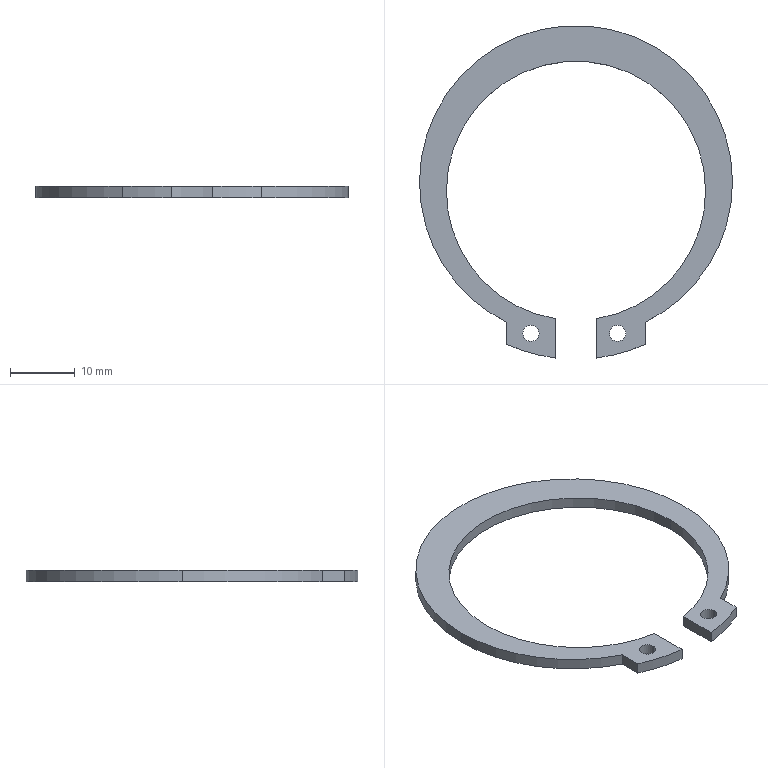Part | STEP file | 10P30 rotor clip | 1 solid | 18 faces | box 48.3 x 51.304 x 1.75 mm | volume 1045 mm3 | cylinder 12 | plane 6 | commonest cylinder face diameters 2.5 x4 40 x3 48.3 x3 52 x2
STEP:
#1=CARTESIAN_POINT('',(0.,0.,0.));
#2=DIRECTION('',(0.,0.,1.));
#3=DIRECTION('',(1.,0.,0.));
#4=AXIS2_PLACEMENT_3D('',#1,#2,#3);
#5=CARTESIAN_POINT('',(5.168,-22.009,1.75));
#6=VERTEX_POINT('',#5);
#7=CARTESIAN_POINT('',(5.168,-22.009,0.));
#8=VERTEX_POINT('',#7);
#9=CARTESIAN_POINT('',(5.168,-22.009,1.75));
#10=DIRECTION('',(0.,0.,-1.));
#11=VECTOR('',#10,1.);
#12=LINE('',#9,#11);
#13=CARTESIAN_POINT('',(6.418,-22.009,1.75));
#14=DIRECTION('',(0.,0.,-1.));
#15=DIRECTION('',(-1.,0.,0.));
#16=AXIS2_PLACEMENT_3D('',#13,#14,#15);
#17=CYLINDRICAL_SURFACE('',#16,1.25);
#18=CARTESIAN_POINT('',(6.283,0.));
#19=DIRECTION('',(0.,1.));
#20=VECTOR('',#19,1.);
#21=LINE('',#18,#20);
#22=(GEOMETRIC_REPRESENTATION_CONTEXT(2)PARAMETRIC_REPRESENTATION_CONTEXT()REPRESENTATION_CONTEXT('',''));
#23=DEFINITIONAL_REPRESENTATION('',(#21),#22);
#24=PCURVE('',#17,#23);
#25=CARTESIAN_POINT('',(6.418,-22.009,1.75));
#26=DIRECTION('',(0.,0.,-1.));
#27=DIRECTION('',(-1.,0.,0.));
#28=AXIS2_PLACEMENT_3D('',#25,#26,#27);
#29=CYLINDRICAL_SURFACE('',#28,1.25);
#30=CARTESIAN_POINT('',(0.,0.));
#31=DIRECTION('',(0.,1.));
#32=VECTOR('',#31,1.);
#33=LINE('',#30,#32);
#34=(GEOMETRIC_REPRESENTATION_CONTEXT(2)PARAMETRIC_REPRESENTATION_CONTEXT()REPRESENTATION_CONTEXT('',''));
#35=DEFINITIONAL_REPRESENTATION('',(#33),#34);
#36=PCURVE('',#29,#35);
#37=SURFACE_CURVE('',#12,(#24,#36),.PCURVE_S1.);
#38=EDGE_CURVE('',#6,#8,#37,.T.);
#39=ORIENTED_EDGE('',*,*,#38,.T.);
#40=CARTESIAN_POINT('',(7.668,-22.009,0.));
#41=VERTEX_POINT('',#40);
#42=CARTESIAN_POINT('',(6.418,-22.009,0.));
#43=DIRECTION('',(0.,0.,1.));
#44=DIRECTION('',(-1.,0.,0.));
#45=AXIS2_PLACEMENT_3D('',#42,#43,#44);
#46=CIRCLE('',#45,1.25);
#47=CARTESIAN_POINT('',(6.283,1.75));
#48=DIRECTION('',(-1.,0.));
#49=VECTOR('',#48,1.);
#50=LINE('',#47,#49);
#51=(GEOMETRIC_REPRESENTATION_CONTEXT(2)PARAMETRIC_REPRESENTATION_CONTEXT()REPRESENTATION_CONTEXT('',''));
#52=DEFINITIONAL_REPRESENTATION('',(#50),#51);
#53=PCURVE('',#17,#52);
#54=CARTESIAN_POINT('',(0.,0.,0.));
#55=DIRECTION('',(0.,0.,1.));
#56=DIRECTION('',(1.,0.,0.));
#57=AXIS2_PLACEMENT_3D('',#54,#55,#56);
#58=PLANE('',#57);
#59=CARTESIAN_POINT('',(6.418,-22.009));
#60=DIRECTION('',(-1.,0.));
#61=AXIS2_PLACEMENT_2D('',#59,#60);
#62=CIRCLE('',#61,1.25);
#63=(GEOMETRIC_REPRESENTATION_CONTEXT(2)PARAMETRIC_REPRESENTATION_CONTEXT()REPRESENTATION_CONTEXT('',''));
#64=DEFINITIONAL_REPRESENTATION('',(#62),#63);
#65=PCURVE('',#58,#64);
#66=SURFACE_CURVE('',#46,(#53,#65),.PCURVE_S1.);
#67=EDGE_CURVE('',#8,#41,#66,.T.);
#68=ORIENTED_EDGE('',*,*,#67,.T.);
#69=CARTESIAN_POINT('',(7.668,-22.009,1.75));
#70=VERTEX_POINT('',#69);
#71=CARTESIAN_POINT('',(7.668,-22.009,1.75));
#72=DIRECTION('',(0.,0.,-1.));
#73=VECTOR('',#72,1.);
#74=LINE('',#71,#73);
#75=CARTESIAN_POINT('',(3.142,0.));
#76=DIRECTION('',(0.,1.));
#77=VECTOR('',#76,1.);
#78=LINE('',#75,#77);
#79=(GEOMETRIC_REPRESENTATION_CONTEXT(2)PARAMETRIC_REPRESENTATION_CONTEXT()REPRESENTATION_CONTEXT('',''));
#80=DEFINITIONAL_REPRESENTATION('',(#78),#79);
#81=PCURVE('',#17,#80);
#82=CARTESIAN_POINT('',(3.142,0.));
#83=DIRECTION('',(0.,1.));
#84=VECTOR('',#83,1.);
#85=LINE('',#82,#84);
#86=(GEOMETRIC_REPRESENTATION_CONTEXT(2)PARAMETRIC_REPRESENTATION_CONTEXT()REPRESENTATION_CONTEXT('',''));
#87=DEFINITIONAL_REPRESENTATION('',(#85),#86);
#88=PCURVE('',#29,#87);
#89=SURFACE_CURVE('',#74,(#81,#88),.PCURVE_S1.);
#90=EDGE_CURVE('',#70,#41,#89,.T.);
#91=ORIENTED_EDGE('',*,*,#90,.F.);
#92=CARTESIAN_POINT('',(6.418,-22.009,1.75));
#93=DIRECTION('',(0.,0.,-1.));
#94=DIRECTION('',(-1.,0.,0.));
#95=AXIS2_PLACEMENT_3D('',#92,#93,#94);
#96=CIRCLE('',#95,1.25);
#97=CARTESIAN_POINT('',(0.,0.));
#98=DIRECTION('',(1.,0.));
#99=VECTOR('',#98,1.);
#100=LINE('',#97,#99);
#101=(GEOMETRIC_REPRESENTATION_CONTEXT(2)PARAMETRIC_REPRESENTATION_CONTEXT()REPRESENTATION_CONTEXT('',''));
#102=DEFINITIONAL_REPRESENTATION('',(#100),#101);
#103=PCURVE('',#17,#102);
#104=CARTESIAN_POINT('',(0.,0.,1.75));
#105=DIRECTION('',(0.,0.,1.));
#106=DIRECTION('',(1.,0.,0.));
#107=AXIS2_PLACEMENT_3D('',#104,#105,#106);
#108=PLANE('',#107);
#109=CARTESIAN_POINT('',(5.168,-22.009));
#110=CARTESIAN_POINT('',(5.168,-19.844));
#111=CARTESIAN_POINT('',(7.043,-20.926));
#112=CARTESIAN_POINT('',(8.918,-22.009));
#113=CARTESIAN_POINT('',(7.043,-23.092));
#114=CARTESIAN_POINT('',(5.168,-24.174));
#115=CARTESIAN_POINT('',(5.168,-22.009));
#116=(BOUNDED_CURVE()B_SPLINE_CURVE(2,(#109,#110,#111,#112,#113,#114,#115),.UNSPECIFIED.,.T.,.F.)B_SPLINE_CURVE_WITH_KNOTS((1,2,2,2,2,1),(-2.094,0.,2.094,4.189,6.283,8.378),.UNSPECIFIED.)CURVE()GEOMETRIC_REPRESENTATION_ITEM()RATIONAL_B_SPLINE_CURVE((1.,0.5,1.,0.5,1.,0.5,1.))REPRESENTATION_ITEM(''));
#117=(GEOMETRIC_REPRESENTATION_CONTEXT(2)PARAMETRIC_REPRESENTATION_CONTEXT()REPRESENTATION_CONTEXT('',''));
#118=DEFINITIONAL_REPRESENTATION('',(#116),#117);
#119=PCURVE('',#108,#118);
#120=SURFACE_CURVE('',#96,(#103,#119),.PCURVE_S1.);
#121=EDGE_CURVE('',#70,#6,#120,.T.);
#122=ORIENTED_EDGE('',*,*,#121,.T.);
#123=EDGE_LOOP('',(#39,#68,#91,#122));
#124=FACE_BOUND('',#123,.F.);
#125=ADVANCED_FACE('',(#124),#17,.F.);
#126=CARTESIAN_POINT('',(24.15,1.35,1.75));
#127=VERTEX_POINT('',#126);
#128=CARTESIAN_POINT('',(-24.15,1.35,1.75));
#129=VERTEX_POINT('',#128);
#130=CARTESIAN_POINT('',(0.,1.35,1.75));
#131=DIRECTION('',(0.,0.,1.));
#132=DIRECTION('',(-1.,0.,0.));
#133=AXIS2_PLACEMENT_3D('',#130,#131,#132);
#134=CIRCLE('',#133,24.15);
#135=CARTESIAN_POINT('',(0.,1.35,1.75));
#136=DIRECTION('',(0.,0.,-1.));
#137=DIRECTION('',(-1.,0.,0.));
#138=AXIS2_PLACEMENT_3D('',#135,#136,#137);
#139=CYLINDRICAL_SURFACE('',#138,24.15);
#140=CARTESIAN_POINT('',(6.283,0.));
#141=DIRECTION('',(-1.,0.));
#142=VECTOR('',#141,1.);
#143=LINE('',#140,#142);
#144=(GEOMETRIC_REPRESENTATION_CONTEXT(2)PARAMETRIC_REPRESENTATION_CONTEXT()REPRESENTATION_CONTEXT('',''));
#145=DEFINITIONAL_REPRESENTATION('',(#143),#144);
#146=PCURVE('',#139,#145);
#147=CARTESIAN_POINT('',(0.,1.35));
#148=DIRECTION('',(-1.,0.));
#149=AXIS2_PLACEMENT_2D('',#147,#148);
#150=CIRCLE('',#149,24.15);
#151=(GEOMETRIC_REPRESENTATION_CONTEXT(2)PARAMETRIC_REPRESENTATION_CONTEXT()REPRESENTATION_CONTEXT('',''));
#152=DEFINITIONAL_REPRESENTATION('',(#150),#151);
#153=PCURVE('',#108,#152);
#154=SURFACE_CURVE('',#134,(#146,#153),.PCURVE_S1.);
#155=EDGE_CURVE('',#127,#129,#154,.T.);
#156=ORIENTED_EDGE('',*,*,#155,.F.);
#157=CARTESIAN_POINT('',(24.15,1.35,0.));
#158=VERTEX_POINT('',#157);
#159=CARTESIAN_POINT('',(24.15,1.35,1.75));
#160=DIRECTION('',(0.,0.,-1.));
#161=VECTOR('',#160,1.);
#162=LINE('',#159,#161);
#163=CARTESIAN_POINT('',(3.142,0.));
#164=DIRECTION('',(0.,1.));
#165=VECTOR('',#164,1.);
#166=LINE('',#163,#165);
#167=(GEOMETRIC_REPRESENTATION_CONTEXT(2)PARAMETRIC_REPRESENTATION_CONTEXT()REPRESENTATION_CONTEXT('',''));
#168=DEFINITIONAL_REPRESENTATION('',(#166),#167);
#169=PCURVE('',#139,#168);
#170=CARTESIAN_POINT('',(0.,1.35,1.75));
#171=DIRECTION('',(0.,0.,-1.));
#172=DIRECTION('',(-1.,0.,0.));
#173=AXIS2_PLACEMENT_3D('',#170,#171,#172);
#174=CYLINDRICAL_SURFACE('',#173,24.15);
#175=CARTESIAN_POINT('',(3.142,0.));
#176=DIRECTION('',(0.,1.));
#177=VECTOR('',#176,1.);
#178=LINE('',#175,#177);
#179=(GEOMETRIC_REPRESENTATION_CONTEXT(2)PARAMETRIC_REPRESENTATION_CONTEXT()REPRESENTATION_CONTEXT('',''));
#180=DEFINITIONAL_REPRESENTATION('',(#178),#179);
#181=PCURVE('',#174,#180);
#182=SURFACE_CURVE('',#162,(#169,#181),.PCURVE_S1.);
#183=EDGE_CURVE('',#127,#158,#182,.T.);
#184=ORIENTED_EDGE('',*,*,#183,.T.);
#185=CARTESIAN_POINT('',(-24.15,1.35,0.));
#186=VERTEX_POINT('',#185);
#187=CARTESIAN_POINT('',(0.,1.35,0.));
#188=DIRECTION('',(0.,0.,1.));
#189=DIRECTION('',(-1.,0.,0.));
#190=AXIS2_PLACEMENT_3D('',#187,#188,#189);
#191=CIRCLE('',#190,24.15);
#192=CARTESIAN_POINT('',(6.283,1.75));
#193=DIRECTION('',(-1.,0.));
#194=VECTOR('',#193,1.);
#195=LINE('',#192,#194);
#196=(GEOMETRIC_REPRESENTATION_CONTEXT(2)PARAMETRIC_REPRESENTATION_CONTEXT()REPRESENTATION_CONTEXT('',''));
#197=DEFINITIONAL_REPRESENTATION('',(#195),#196);
#198=PCURVE('',#139,#197);
#199=CARTESIAN_POINT('',(0.,1.35));
#200=DIRECTION('',(-1.,0.));
#201=AXIS2_PLACEMENT_2D('',#199,#200);
#202=CIRCLE('',#201,24.15);
#203=(GEOMETRIC_REPRESENTATION_CONTEXT(2)PARAMETRIC_REPRESENTATION_CONTEXT()REPRESENTATION_CONTEXT('',''));
#204=DEFINITIONAL_REPRESENTATION('',(#202),#203);
#205=PCURVE('',#58,#204);
#206=SURFACE_CURVE('',#191,(#198,#205),.PCURVE_S1.);
#207=EDGE_CURVE('',#158,#186,#206,.T.);
#208=ORIENTED_EDGE('',*,*,#207,.T.);
#209=CARTESIAN_POINT('',(-24.15,1.35,1.75));
#210=DIRECTION('',(0.,0.,-1.));
#211=VECTOR('',#210,1.);
#212=LINE('',#209,#211);
#213=CARTESIAN_POINT('',(0.,0.));
#214=DIRECTION('',(0.,1.));
#215=VECTOR('',#214,1.);
#216=LINE('',#213,#215);
#217=(GEOMETRIC_REPRESENTATION_CONTEXT(2)PARAMETRIC_REPRESENTATION_CONTEXT()REPRESENTATION_CONTEXT('',''));
#218=DEFINITIONAL_REPRESENTATION('',(#216),#217);
#219=PCURVE('',#139,#218);
#220=CARTESIAN_POINT('',(0.,1.35,1.75));
#221=DIRECTION('',(0.,0.,-1.));
#222=DIRECTION('',(-1.,0.,0.));
#223=AXIS2_PLACEMENT_3D('',#220,#221,#222);
#224=CYLINDRICAL_SURFACE('',#223,24.15);
#225=CARTESIAN_POINT('',(6.283,0.));
#226=DIRECTION('',(0.,1.));
#227=VECTOR('',#226,1.);
#228=LINE('',#225,#227);
#229=(GEOMETRIC_REPRESENTATION_CONTEXT(2)PARAMETRIC_REPRESENTATION_CONTEXT()REPRESENTATION_CONTEXT('',''));
#230=DEFINITIONAL_REPRESENTATION('',(#228),#229);
#231=PCURVE('',#224,#230);
#232=SURFACE_CURVE('',#212,(#219,#231),.PCURVE_S1.);
#233=EDGE_CURVE('',#129,#186,#232,.T.);
#234=ORIENTED_EDGE('',*,*,#233,.F.);
#235=EDGE_LOOP('',(#156,#184,#208,#234));
#236=FACE_BOUND('',#235,.T.);
#237=ADVANCED_FACE('',(#236),#139,.T.);
#238=CARTESIAN_POINT('',(-10.718,-20.291,1.75));
#239=VERTEX_POINT('',#238);
#240=CARTESIAN_POINT('',(0.,1.35,1.75));
#241=DIRECTION('',(0.,0.,1.));
#242=DIRECTION('',(-1.,0.,0.));
#243=AXIS2_PLACEMENT_3D('',#240,#241,#242);
#244=CIRCLE('',#243,24.15);
#245=CARTESIAN_POINT('',(6.283,0.));
#246=DIRECTION('',(-1.,0.));
#247=VECTOR('',#246,1.);
#248=LINE('',#245,#247);
#249=(GEOMETRIC_REPRESENTATION_CONTEXT(2)PARAMETRIC_REPRESENTATION_CONTEXT()REPRESENTATION_CONTEXT('',''));
#250=DEFINITIONAL_REPRESENTATION('',(#248),#249);
#251=PCURVE('',#224,#250);
#252=CARTESIAN_POINT('',(0.,1.35));
#253=DIRECTION('',(-1.,0.));
#254=AXIS2_PLACEMENT_2D('',#252,#253);
#255=CIRCLE('',#254,24.15);
#256=(GEOMETRIC_REPRESENTATION_CONTEXT(2)PARAMETRIC_REPRESENTATION_CONTEXT()REPRESENTATION_CONTEXT('',''));
#257=DEFINITIONAL_REPRESENTATION('',(#255),#256);
#258=PCURVE('',#108,#257);
#259=SURFACE_CURVE('',#244,(#251,#258),.PCURVE_S1.);
#260=EDGE_CURVE('',#129,#239,#259,.T.);
#261=ORIENTED_EDGE('',*,*,#260,.F.);
#262=ORIENTED_EDGE('',*,*,#233,.T.);
#263=CARTESIAN_POINT('',(-10.718,-20.291,0.));
#264=VERTEX_POINT('',#263);
#265=CARTESIAN_POINT('',(0.,1.35,0.));
#266=DIRECTION('',(0.,0.,1.));
#267=DIRECTION('',(-1.,0.,0.));
#268=AXIS2_PLACEMENT_3D('',#265,#266,#267);
#269=CIRCLE('',#268,24.15);
#270=CARTESIAN_POINT('',(6.283,1.75));
#271=DIRECTION('',(-1.,0.));
#272=VECTOR('',#271,1.);
#273=LINE('',#270,#272);
#274=(GEOMETRIC_REPRESENTATION_CONTEXT(2)PARAMETRIC_REPRESENTATION_CONTEXT()REPRESENTATION_CONTEXT('',''));
#275=DEFINITIONAL_REPRESENTATION('',(#273),#274);
#276=PCURVE('',#224,#275);
#277=CARTESIAN_POINT('',(0.,1.35));
#278=DIRECTION('',(-1.,0.));
#279=AXIS2_PLACEMENT_2D('',#277,#278);
#280=CIRCLE('',#279,24.15);
#281=(GEOMETRIC_REPRESENTATION_CONTEXT(2)PARAMETRIC_REPRESENTATION_CONTEXT()REPRESENTATION_CONTEXT('',''));
#282=DEFINITIONAL_REPRESENTATION('',(#280),#281);
#283=PCURVE('',#58,#282);
#284=SURFACE_CURVE('',#269,(#276,#283),.PCURVE_S1.);
#285=EDGE_CURVE('',#186,#264,#284,.T.);
#286=ORIENTED_EDGE('',*,*,#285,.T.);
#287=CARTESIAN_POINT('',(-10.718,-20.291,1.75));
#288=DIRECTION('',(0.,0.,1.));
#289=VECTOR('',#288,1.);
#290=LINE('',#287,#289);
#291=CARTESIAN_POINT('',(5.172,0.));
#292=DIRECTION('',(0.,-1.));
#293=VECTOR('',#292,1.);
#294=LINE('',#291,#293);
#295=(GEOMETRIC_REPRESENTATION_CONTEXT(2)PARAMETRIC_REPRESENTATION_CONTEXT()REPRESENTATION_CONTEXT('',''));
#296=DEFINITIONAL_REPRESENTATION('',(#294),#295);
#297=PCURVE('',#224,#296);
#298=CARTESIAN_POINT('',(-10.718,-23.688,1.75));
#299=DIRECTION('',(1.,0.,0.));
#300=DIRECTION('',(0.,0.,-1.));
#301=AXIS2_PLACEMENT_3D('',#298,#299,#300);
#302=PLANE('',#301);
#303=CARTESIAN_POINT('',(0.,3.397));
#304=DIRECTION('',(-1.,0.));
#305=VECTOR('',#304,1.);
#306=LINE('',#303,#305);
#307=(GEOMETRIC_REPRESENTATION_CONTEXT(2)PARAMETRIC_REPRESENTATION_CONTEXT()REPRESENTATION_CONTEXT('',''));
#308=DEFINITIONAL_REPRESENTATION('',(#306),#307);
#309=PCURVE('',#302,#308);
#310=SURFACE_CURVE('',#290,(#297,#309),.PCURVE_S1.);
#311=EDGE_CURVE('',#264,#239,#310,.T.);
#312=ORIENTED_EDGE('',*,*,#311,.T.);
#313=EDGE_LOOP('',(#261,#262,#286,#312));
#314=FACE_BOUND('',#313,.T.);
#315=ADVANCED_FACE('',(#314),#224,.T.);
#316=CARTESIAN_POINT('',(3.185,-19.745,0.));
#317=VERTEX_POINT('',#316);
#318=CARTESIAN_POINT('',(3.185,-19.745,1.75));
#319=VERTEX_POINT('',#318);
#320=CARTESIAN_POINT('',(3.185,-19.745,1.75));
#321=DIRECTION('',(0.,0.,1.));
#322=VECTOR('',#321,1.);
#323=LINE('',#320,#322);
#324=CARTESIAN_POINT('',(0.,0.,1.75));
#325=DIRECTION('',(0.,0.,-1.));
#326=DIRECTION('',(-1.,0.,0.));
#327=AXIS2_PLACEMENT_3D('',#324,#325,#326);
#328=CYLINDRICAL_SURFACE('',#327,20.);
#329=CARTESIAN_POINT('',(4.552,0.));
#330=DIRECTION('',(0.,-1.));
#331=VECTOR('',#330,1.);
#332=LINE('',#329,#331);
#333=(GEOMETRIC_REPRESENTATION_CONTEXT(2)PARAMETRIC_REPRESENTATION_CONTEXT()REPRESENTATION_CONTEXT('',''));
#334=DEFINITIONAL_REPRESENTATION('',(#332),#333);
#335=PCURVE('',#328,#334);
#336=CARTESIAN_POINT('',(3.185,-25.804,1.75));
#337=DIRECTION('',(1.,0.,0.));
#338=DIRECTION('',(0.,0.,-1.));
#339=AXIS2_PLACEMENT_3D('',#336,#337,#338);
#340=PLANE('',#339);
#341=CARTESIAN_POINT('',(0.,6.059));
#342=DIRECTION('',(-1.,0.));
#343=VECTOR('',#342,1.);
#344=LINE('',#341,#343);
#345=(GEOMETRIC_REPRESENTATION_CONTEXT(2)PARAMETRIC_REPRESENTATION_CONTEXT()REPRESENTATION_CONTEXT('',''));
#346=DEFINITIONAL_REPRESENTATION('',(#344),#345);
#347=PCURVE('',#340,#346);
#348=SURFACE_CURVE('',#323,(#335,#347),.PCURVE_S1.);
#349=EDGE_CURVE('',#317,#319,#348,.T.);
#350=ORIENTED_EDGE('',*,*,#349,.F.);
#351=CARTESIAN_POINT('',(20.,0.,0.));
#352=VERTEX_POINT('',#351);
#353=CARTESIAN_POINT('',(0.,0.,0.));
#354=DIRECTION('',(0.,0.,1.));
#355=DIRECTION('',(-1.,0.,0.));
#356=AXIS2_PLACEMENT_3D('',#353,#354,#355);
#357=CIRCLE('',#356,20.);
#358=CARTESIAN_POINT('',(6.283,1.75));
#359=DIRECTION('',(-1.,0.));
#360=VECTOR('',#359,1.);
#361=LINE('',#358,#360);
#362=(GEOMETRIC_REPRESENTATION_CONTEXT(2)PARAMETRIC_REPRESENTATION_CONTEXT()REPRESENTATION_CONTEXT('',''));
#363=DEFINITIONAL_REPRESENTATION('',(#361),#362);
#364=PCURVE('',#328,#363);
#365=CARTESIAN_POINT('',(0.,0.));
#366=DIRECTION('',(-1.,0.));
#367=AXIS2_PLACEMENT_2D('',#365,#366);
#368=CIRCLE('',#367,20.);
#369=(GEOMETRIC_REPRESENTATION_CONTEXT(2)PARAMETRIC_REPRESENTATION_CONTEXT()REPRESENTATION_CONTEXT('',''));
#370=DEFINITIONAL_REPRESENTATION('',(#368),#369);
#371=PCURVE('',#58,#370);
#372=SURFACE_CURVE('',#357,(#364,#371),.PCURVE_S1.);
#373=EDGE_CURVE('',#317,#352,#372,.T.);
#374=ORIENTED_EDGE('',*,*,#373,.T.);
#375=CARTESIAN_POINT('',(20.,0.,1.75));
#376=VERTEX_POINT('',#375);
#377=CARTESIAN_POINT('',(20.,0.,1.75));
#378=DIRECTION('',(0.,0.,-1.));
#379=VECTOR('',#378,1.);
#380=LINE('',#377,#379);
#381=CARTESIAN_POINT('',(3.142,0.));
#382=DIRECTION('',(0.,1.));
#383=VECTOR('',#382,1.);
#384=LINE('',#381,#383);
#385=(GEOMETRIC_REPRESENTATION_CONTEXT(2)PARAMETRIC_REPRESENTATION_CONTEXT()REPRESENTATION_CONTEXT('',''));
#386=DEFINITIONAL_REPRESENTATION('',(#384),#385);
#387=PCURVE('',#328,#386);
#388=CARTESIAN_POINT('',(0.,0.,1.75));
#389=DIRECTION('',(0.,0.,-1.));
#390=DIRECTION('',(-1.,0.,0.));
#391=AXIS2_PLACEMENT_3D('',#388,#389,#390);
#392=CYLINDRICAL_SURFACE('',#391,20.);
#393=CARTESIAN_POINT('',(3.142,0.));
#394=DIRECTION('',(0.,1.));
#395=VECTOR('',#394,1.);
#396=LINE('',#393,#395);
#397=(GEOMETRIC_REPRESENTATION_CONTEXT(2)PARAMETRIC_REPRESENTATION_CONTEXT()REPRESENTATION_CONTEXT('',''));
#398=DEFINITIONAL_REPRESENTATION('',(#396),#397);
#399=PCURVE('',#392,#398);
#400=SURFACE_CURVE('',#380,(#387,#399),.PCURVE_S1.);
#401=EDGE_CURVE('',#376,#352,#400,.T.);
#402=ORIENTED_EDGE('',*,*,#401,.F.);
#403=CARTESIAN_POINT('',(0.,0.,1.75));
#404=DIRECTION('',(0.,0.,-1.));
#405=DIRECTION('',(-1.,0.,0.));
#406=AXIS2_PLACEMENT_3D('',#403,#404,#405);
#407=CIRCLE('',#406,20.);
#408=CARTESIAN_POINT('',(0.,0.));
#409=DIRECTION('',(1.,0.));
#410=VECTOR('',#409,1.);
#411=LINE('',#408,#410);
#412=(GEOMETRIC_REPRESENTATION_CONTEXT(2)PARAMETRIC_REPRESENTATION_CONTEXT()REPRESENTATION_CONTEXT('',''));
#413=DEFINITIONAL_REPRESENTATION('',(#411),#412);
#414=PCURVE('',#328,#413);
#415=CARTESIAN_POINT('',(-20.,0.));
#416=CARTESIAN_POINT('',(-20.,34.641));
#417=CARTESIAN_POINT('',(10.,17.321));
#418=CARTESIAN_POINT('',(40.,0.));
#419=CARTESIAN_POINT('',(10.,-17.321));
#420=CARTESIAN_POINT('',(-20.,-34.641));
#421=CARTESIAN_POINT('',(-20.,0.));
#422=(BOUNDED_CURVE()B_SPLINE_CURVE(2,(#415,#416,#417,#418,#419,#420,#421),.UNSPECIFIED.,.T.,.F.)B_SPLINE_CURVE_WITH_KNOTS((1,2,2,2,2,1),(-2.094,0.,2.094,4.189,6.283,8.378),.UNSPECIFIED.)CURVE()GEOMETRIC_REPRESENTATION_ITEM()RATIONAL_B_SPLINE_CURVE((1.,0.5,1.,0.5,1.,0.5,1.))REPRESENTATION_ITEM(''));
#423=(GEOMETRIC_REPRESENTATION_CONTEXT(2)PARAMETRIC_REPRESENTATION_CONTEXT()REPRESENTATION_CONTEXT('',''));
#424=DEFINITIONAL_REPRESENTATION('',(#422),#423);
#425=PCURVE('',#108,#424);
#426=SURFACE_CURVE('',#407,(#414,#425),.PCURVE_S1.);
#427=EDGE_CURVE('',#376,#319,#426,.T.);
#428=ORIENTED_EDGE('',*,*,#427,.T.);
#429=EDGE_LOOP('',(#350,#374,#402,#428));
#430=FACE_BOUND('',#429,.F.);
#431=ADVANCED_FACE('',(#430),#328,.F.);
#432=CARTESIAN_POINT('',(-20.,0.,0.));
#433=VERTEX_POINT('',#432);
#434=CARTESIAN_POINT('',(0.,0.,0.));
#435=DIRECTION('',(0.,0.,1.));
#436=DIRECTION('',(-1.,0.,0.));
#437=AXIS2_PLACEMENT_3D('',#434,#435,#436);
#438=CIRCLE('',#437,20.);
#439=CARTESIAN_POINT('',(6.283,1.75));
#440=DIRECTION('',(-1.,0.));
#441=VECTOR('',#440,1.);
#442=LINE('',#439,#441);
#443=(GEOMETRIC_REPRESENTATION_CONTEXT(2)PARAMETRIC_REPRESENTATION_CONTEXT()REPRESENTATION_CONTEXT('',''));
#444=DEFINITIONAL_REPRESENTATION('',(#442),#443);
#445=PCURVE('',#392,#444);
#446=CARTESIAN_POINT('',(0.,0.));
#447=DIRECTION('',(-1.,0.));
#448=AXIS2_PLACEMENT_2D('',#446,#447);
#449=CIRCLE('',#448,20.);
#450=(GEOMETRIC_REPRESENTATION_CONTEXT(2)PARAMETRIC_REPRESENTATION_CONTEXT()REPRESENTATION_CONTEXT('',''));
#451=DEFINITIONAL_REPRESENTATION('',(#449),#450);
#452=PCURVE('',#58,#451);
#453=SURFACE_CURVE('',#438,(#445,#452),.PCURVE_S1.);
#454=EDGE_CURVE('',#352,#433,#453,.T.);
#455=ORIENTED_EDGE('',*,*,#454,.T.);
#456=CARTESIAN_POINT('',(-20.,0.,1.75));
#457=VERTEX_POINT('',#456);
#458=CARTESIAN_POINT('',(-20.,0.,1.75));
#459=DIRECTION('',(0.,0.,-1.));
#460=VECTOR('',#459,1.);
#461=LINE('',#458,#460);
#462=CARTESIAN_POINT('',(0.,0.));
#463=DIRECTION('',(0.,1.));
#464=VECTOR('',#463,1.);
#465=LINE('',#462,#464);
#466=(GEOMETRIC_REPRESENTATION_CONTEXT(2)PARAMETRIC_REPRESENTATION_CONTEXT()REPRESENTATION_CONTEXT('',''));
#467=DEFINITIONAL_REPRESENTATION('',(#465),#466);
#468=PCURVE('',#392,#467);
#469=CARTESIAN_POINT('',(0.,0.,1.75));
#470=DIRECTION('',(0.,0.,-1.));
#471=DIRECTION('',(-1.,0.,0.));
#472=AXIS2_PLACEMENT_3D('',#469,#470,#471);
#473=CYLINDRICAL_SURFACE('',#472,20.);
#474=CARTESIAN_POINT('',(6.283,0.));
#475=DIRECTION('',(0.,1.));
#476=VECTOR('',#475,1.);
#477=LINE('',#474,#476);
#478=(GEOMETRIC_REPRESENTATION_CONTEXT(2)PARAMETRIC_REPRESENTATION_CONTEXT()REPRESENTATION_CONTEXT('',''));
#479=DEFINITIONAL_REPRESENTATION('',(#477),#478);
#480=PCURVE('',#473,#479);
#481=SURFACE_CURVE('',#461,(#468,#480),.PCURVE_S1.);
#482=EDGE_CURVE('',#457,#433,#481,.T.);
#483=ORIENTED_EDGE('',*,*,#482,.F.);
#484=CARTESIAN_POINT('',(0.,0.,1.75));
#485=DIRECTION('',(0.,0.,-1.));
#486=DIRECTION('',(-1.,0.,0.));
#487=AXIS2_PLACEMENT_3D('',#484,#485,#486);
#488=CIRCLE('',#487,20.);
#489=CARTESIAN_POINT('',(0.,0.));
#490=DIRECTION('',(1.,0.));
#491=VECTOR('',#490,1.);
#492=LINE('',#489,#491);
#493=(GEOMETRIC_REPRESENTATION_CONTEXT(2)PARAMETRIC_REPRESENTATION_CONTEXT()REPRESENTATION_CONTEXT('',''));
#494=DEFINITIONAL_REPRESENTATION('',(#492),#493);
#495=PCURVE('',#392,#494);
#496=CARTESIAN_POINT('',(-20.,0.));
#497=CARTESIAN_POINT('',(-20.,34.641));
#498=CARTESIAN_POINT('',(10.,17.321));
#499=CARTESIAN_POINT('',(40.,0.));
#500=CARTESIAN_POINT('',(10.,-17.321));
#501=CARTESIAN_POINT('',(-20.,-34.641));
#502=CARTESIAN_POINT('',(-20.,0.));
#503=(BOUNDED_CURVE()B_SPLINE_CURVE(2,(#496,#497,#498,#499,#500,#501,#502),.UNSPECIFIED.,.T.,.F.)B_SPLINE_CURVE_WITH_KNOTS((1,2,2,2,2,1),(-2.094,0.,2.094,4.189,6.283,8.378),.UNSPECIFIED.)CURVE()GEOMETRIC_REPRESENTATION_ITEM()RATIONAL_B_SPLINE_CURVE((1.,0.5,1.,0.5,1.,0.5,1.))REPRESENTATION_ITEM(''));
#504=(GEOMETRIC_REPRESENTATION_CONTEXT(2)PARAMETRIC_REPRESENTATION_CONTEXT()REPRESENTATION_CONTEXT('',''));
#505=DEFINITIONAL_REPRESENTATION('',(#503),#504);
#506=PCURVE('',#108,#505);
#507=SURFACE_CURVE('',#488,(#495,#506),.PCURVE_S1.);
#508=EDGE_CURVE('',#457,#376,#507,.T.);
#509=ORIENTED_EDGE('',*,*,#508,.T.);
#510=ORIENTED_EDGE('',*,*,#401,.T.);
#511=EDGE_LOOP('',(#455,#483,#509,#510));
#512=FACE_BOUND('',#511,.F.);
#513=ADVANCED_FACE('',(#512),#392,.F.);
#514=CARTESIAN_POINT('',(-8.204,-22.009,1.75));
#515=VERTEX_POINT('',#514);
#516=CARTESIAN_POINT('',(-8.204,-22.009,0.));
#517=VERTEX_POINT('',#516);
#518=CARTESIAN_POINT('',(-8.204,-22.009,1.75));
#519=DIRECTION('',(0.,0.,-1.));
#520=VECTOR('',#519,1.);
#521=LINE('',#518,#520);
#522=CARTESIAN_POINT('',(-6.954,-22.009,1.75));
#523=DIRECTION('',(0.,0.,-1.));
#524=DIRECTION('',(-1.,0.,0.));
#525=AXIS2_PLACEMENT_3D('',#522,#523,#524);
#526=CYLINDRICAL_SURFACE('',#525,1.25);
#527=CARTESIAN_POINT('',(6.283,0.));
#528=DIRECTION('',(0.,1.));
#529=VECTOR('',#528,1.);
#530=LINE('',#527,#529);
#531=(GEOMETRIC_REPRESENTATION_CONTEXT(2)PARAMETRIC_REPRESENTATION_CONTEXT()REPRESENTATION_CONTEXT('',''));
#532=DEFINITIONAL_REPRESENTATION('',(#530),#531);
#533=PCURVE('',#526,#532);
#534=CARTESIAN_POINT('',(-6.954,-22.009,1.75));
#535=DIRECTION('',(0.,0.,-1.));
#536=DIRECTION('',(-1.,0.,0.));
#537=AXIS2_PLACEMENT_3D('',#534,#535,#536);
#538=CYLINDRICAL_SURFACE('',#537,1.25);
#539=CARTESIAN_POINT('',(0.,0.));
#540=DIRECTION('',(0.,1.));
#541=VECTOR('',#540,1.);
#542=LINE('',#539,#541);
#543=(GEOMETRIC_REPRESENTATION_CONTEXT(2)PARAMETRIC_REPRESENTATION_CONTEXT()REPRESENTATION_CONTEXT('',''));
#544=DEFINITIONAL_REPRESENTATION('',(#542),#543);
#545=PCURVE('',#538,#544);
#546=SURFACE_CURVE('',#521,(#533,#545),.PCURVE_S1.);
#547=EDGE_CURVE('',#515,#517,#546,.T.);
#548=ORIENTED_EDGE('',*,*,#547,.T.);
#549=CARTESIAN_POINT('',(-5.704,-22.009,0.));
#550=VERTEX_POINT('',#549);
#551=CARTESIAN_POINT('',(-6.954,-22.009,0.));
#552=DIRECTION('',(0.,0.,1.));
#553=DIRECTION('',(-1.,0.,0.));
#554=AXIS2_PLACEMENT_3D('',#551,#552,#553);
#555=CIRCLE('',#554,1.25);
#556=CARTESIAN_POINT('',(6.283,1.75));
#557=DIRECTION('',(-1.,0.));
#558=VECTOR('',#557,1.);
#559=LINE('',#556,#558);
#560=(GEOMETRIC_REPRESENTATION_CONTEXT(2)PARAMETRIC_REPRESENTATION_CONTEXT()REPRESENTATION_CONTEXT('',''));
#561=DEFINITIONAL_REPRESENTATION('',(#559),#560);
#562=PCURVE('',#526,#561);
#563=CARTESIAN_POINT('',(-6.954,-22.009));
#564=DIRECTION('',(-1.,0.));
#565=AXIS2_PLACEMENT_2D('',#563,#564);
#566=CIRCLE('',#565,1.25);
#567=(GEOMETRIC_REPRESENTATION_CONTEXT(2)PARAMETRIC_REPRESENTATION_CONTEXT()REPRESENTATION_CONTEXT('',''));
#568=DEFINITIONAL_REPRESENTATION('',(#566),#567);
#569=PCURVE('',#58,#568);
#570=SURFACE_CURVE('',#555,(#562,#569),.PCURVE_S1.);
#571=EDGE_CURVE('',#517,#550,#570,.T.);
#572=ORIENTED_EDGE('',*,*,#571,.T.);
#573=CARTESIAN_POINT('',(-5.704,-22.009,1.75));
#574=VERTEX_POINT('',#573);
#575=CARTESIAN_POINT('',(-5.704,-22.009,1.75));
#576=DIRECTION('',(0.,0.,-1.));
#577=VECTOR('',#576,1.);
#578=LINE('',#575,#577);
#579=CARTESIAN_POINT('',(3.142,0.));
#580=DIRECTION('',(0.,1.));
#581=VECTOR('',#580,1.);
#582=LINE('',#579,#581);
#583=(GEOMETRIC_REPRESENTATION_CONTEXT(2)PARAMETRIC_REPRESENTATION_CONTEXT()REPRESENTATION_CONTEXT('',''));
#584=DEFINITIONAL_REPRESENTATION('',(#582),#583);
#585=PCURVE('',#526,#584);
#586=CARTESIAN_POINT('',(3.142,0.));
#587=DIRECTION('',(0.,1.));
#588=VECTOR('',#587,1.);
#589=LINE('',#586,#588);
#590=(GEOMETRIC_REPRESENTATION_CONTEXT(2)PARAMETRIC_REPRESENTATION_CONTEXT()REPRESENTATION_CONTEXT('',''));
#591=DEFINITIONAL_REPRESENTATION('',(#589),#590);
#592=PCURVE('',#538,#591);
#593=SURFACE_CURVE('',#578,(#585,#592),.PCURVE_S1.);
#594=EDGE_CURVE('',#574,#550,#593,.T.);
#595=ORIENTED_EDGE('',*,*,#594,.F.);
#596=CARTESIAN_POINT('',(-6.954,-22.009,1.75));
#597=DIRECTION('',(0.,0.,-1.));
#598=DIRECTION('',(-1.,0.,0.));
#599=AXIS2_PLACEMENT_3D('',#596,#597,#598);
#600=CIRCLE('',#599,1.25);
#601=CARTESIAN_POINT('',(0.,0.));
#602=DIRECTION('',(1.,0.));
#603=VECTOR('',#602,1.);
#604=LINE('',#601,#603);
#605=(GEOMETRIC_REPRESENTATION_CONTEXT(2)PARAMETRIC_REPRESENTATION_CONTEXT()REPRESENTATION_CONTEXT('',''));
#606=DEFINITIONAL_REPRESENTATION('',(#604),#605);
#607=PCURVE('',#526,#606);
#608=CARTESIAN_POINT('',(-8.204,-22.009));
#609=CARTESIAN_POINT('',(-8.204,-19.844));
#610=CARTESIAN_POINT('',(-6.329,-20.926));
#611=CARTESIAN_POINT('',(-4.454,-22.009));
#612=CARTESIAN_POINT('',(-6.329,-23.092));
#613=CARTESIAN_POINT('',(-8.204,-24.174));
#614=CARTESIAN_POINT('',(-8.204,-22.009));
#615=(BOUNDED_CURVE()B_SPLINE_CURVE(2,(#608,#609,#610,#611,#612,#613,#614),.UNSPECIFIED.,.T.,.F.)B_SPLINE_CURVE_WITH_KNOTS((1,2,2,2,2,1),(-2.094,0.,2.094,4.189,6.283,8.378),.UNSPECIFIED.)CURVE()GEOMETRIC_REPRESENTATION_ITEM()RATIONAL_B_SPLINE_CURVE((1.,0.5,1.,0.5,1.,0.5,1.))REPRESENTATION_ITEM(''));
#616=(GEOMETRIC_REPRESENTATION_CONTEXT(2)PARAMETRIC_REPRESENTATION_CONTEXT()REPRESENTATION_CONTEXT('',''));
#617=DEFINITIONAL_REPRESENTATION('',(#615),#616);
#618=PCURVE('',#108,#617);
#619=SURFACE_CURVE('',#600,(#607,#618),.PCURVE_S1.);
#620=EDGE_CURVE('',#574,#515,#619,.T.);
#621=ORIENTED_EDGE('',*,*,#620,.T.);
#622=EDGE_LOOP('',(#548,#572,#595,#621));
#623=FACE_BOUND('',#622,.F.);
#624=ADVANCED_FACE('',(#623),#526,.F.);
#625=CARTESIAN_POINT('',(6.418,-22.009,1.75));
#626=DIRECTION('',(0.,0.,-1.));
#627=DIRECTION('',(-1.,0.,0.));
#628=AXIS2_PLACEMENT_3D('',#625,#626,#627);
#629=CIRCLE('',#628,1.25);
#630=CARTESIAN_POINT('',(5.168,-22.009));
#631=CARTESIAN_POINT('',(5.168,-19.844));
#632=CARTESIAN_POINT('',(7.043,-20.926));
#633=CARTESIAN_POINT('',(8.918,-22.009));
#634=CARTESIAN_POINT('',(7.043,-23.092));
#635=CARTESIAN_POINT('',(5.168,-24.174));
#636=CARTESIAN_POINT('',(5.168,-22.009));
#637=(BOUNDED_CURVE()B_SPLINE_CURVE(2,(#630,#631,#632,#633,#634,#635,#636),.UNSPECIFIED.,.T.,.F.)B_SPLINE_CURVE_WITH_KNOTS((1,2,2,2,2,1),(-2.094,0.,2.094,4.189,6.283,8.378),.UNSPECIFIED.)CURVE()GEOMETRIC_REPRESENTATION_ITEM()RATIONAL_B_SPLINE_CURVE((1.,0.5,1.,0.5,1.,0.5,1.))REPRESENTATION_ITEM(''));
#638=(GEOMETRIC_REPRESENTATION_CONTEXT(2)PARAMETRIC_REPRESENTATION_CONTEXT()REPRESENTATION_CONTEXT('',''));
#639=DEFINITIONAL_REPRESENTATION('',(#637),#638);
#640=PCURVE('',#108,#639);
#641=CARTESIAN_POINT('',(0.,0.));
#642=DIRECTION('',(1.,0.));
#643=VECTOR('',#642,1.);
#644=LINE('',#641,#643);
#645=(GEOMETRIC_REPRESENTATION_CONTEXT(2)PARAMETRIC_REPRESENTATION_CONTEXT()REPRESENTATION_CONTEXT('',''));
#646=DEFINITIONAL_REPRESENTATION('',(#644),#645);
#647=PCURVE('',#29,#646);
#648=SURFACE_CURVE('',#629,(#640,#647),.PCURVE_S1.);
#649=EDGE_CURVE('',#6,#70,#648,.T.);
#650=ORIENTED_EDGE('',*,*,#649,.T.);
#651=ORIENTED_EDGE('',*,*,#121,.T.);
#652=EDGE_LOOP('',(#650,#651));
#653=FACE_BOUND('',#652,.T.);
#654=CARTESIAN_POINT('',(10.718,-20.291,1.75));
#655=VERTEX_POINT('',#654);
#656=CARTESIAN_POINT('',(0.,1.35,1.75));
#657=DIRECTION('',(0.,0.,1.));
#658=DIRECTION('',(-1.,0.,0.));
#659=AXIS2_PLACEMENT_3D('',#656,#657,#658);
#660=CIRCLE('',#659,24.15);
#661=CARTESIAN_POINT('',(0.,1.35));
#662=DIRECTION('',(-1.,0.));
#663=AXIS2_PLACEMENT_2D('',#661,#662);
#664=CIRCLE('',#663,24.15);
#665=(GEOMETRIC_REPRESENTATION_CONTEXT(2)PARAMETRIC_REPRESENTATION_CONTEXT()REPRESENTATION_CONTEXT('',''));
#666=DEFINITIONAL_REPRESENTATION('',(#664),#665);
#667=PCURVE('',#108,#666);
#668=CARTESIAN_POINT('',(6.283,0.));
#669=DIRECTION('',(-1.,0.));
#670=VECTOR('',#669,1.);
#671=LINE('',#668,#670);
#672=(GEOMETRIC_REPRESENTATION_CONTEXT(2)PARAMETRIC_REPRESENTATION_CONTEXT()REPRESENTATION_CONTEXT('',''));
#673=DEFINITIONAL_REPRESENTATION('',(#671),#672);
#674=PCURVE('',#174,#673);
#675=SURFACE_CURVE('',#660,(#667,#674),.PCURVE_S1.);
#676=EDGE_CURVE('',#655,#127,#675,.T.);
#677=ORIENTED_EDGE('',*,*,#676,.T.);
#678=ORIENTED_EDGE('',*,*,#155,.T.);
#679=ORIENTED_EDGE('',*,*,#260,.T.);
#680=CARTESIAN_POINT('',(-10.718,-23.688,1.75));
#681=VERTEX_POINT('',#680);
#682=CARTESIAN_POINT('',(-10.718,0.,1.75));
#683=DIRECTION('',(0.,-1.,0.));
#684=VECTOR('',#683,1.);
#685=LINE('',#682,#684);
#686=CARTESIAN_POINT('',(-10.718,0.));
#687=DIRECTION('',(0.,-1.));
#688=VECTOR('',#687,1.);
#689=LINE('',#686,#688);
#690=(GEOMETRIC_REPRESENTATION_CONTEXT(2)PARAMETRIC_REPRESENTATION_CONTEXT()REPRESENTATION_CONTEXT('',''));
#691=DEFINITIONAL_REPRESENTATION('',(#689),#690);
#692=PCURVE('',#108,#691);
#693=CARTESIAN_POINT('',(0.,23.688));
#694=DIRECTION('',(0.,-1.));
#695=VECTOR('',#694,1.);
#696=LINE('',#693,#695);
#697=(GEOMETRIC_REPRESENTATION_CONTEXT(2)PARAMETRIC_REPRESENTATION_CONTEXT()REPRESENTATION_CONTEXT('',''));
#698=DEFINITIONAL_REPRESENTATION('',(#696),#697);
#699=PCURVE('',#302,#698);
#700=SURFACE_CURVE('',#685,(#692,#699),.PCURVE_S1.);
#701=EDGE_CURVE('',#239,#681,#700,.T.);
#702=ORIENTED_EDGE('',*,*,#701,.T.);
#703=CARTESIAN_POINT('',(-3.185,-25.804,1.75));
#704=VERTEX_POINT('',#703);
#705=CARTESIAN_POINT('',(0.,0.,1.75));
#706=DIRECTION('',(0.,0.,1.));
#707=DIRECTION('',(-1.,0.,0.));
#708=AXIS2_PLACEMENT_3D('',#705,#706,#707);
#709=CIRCLE('',#708,26.);
#710=CARTESIAN_POINT('',(0.,0.));
#711=DIRECTION('',(-1.,0.));
#712=AXIS2_PLACEMENT_2D('',#710,#711);
#713=CIRCLE('',#712,26.);
#714=(GEOMETRIC_REPRESENTATION_CONTEXT(2)PARAMETRIC_REPRESENTATION_CONTEXT()REPRESENTATION_CONTEXT('',''));
#715=DEFINITIONAL_REPRESENTATION('',(#713),#714);
#716=PCURVE('',#108,#715);
#717=CARTESIAN_POINT('',(0.,0.,1.75));
#718=DIRECTION('',(0.,0.,-1.));
#719=DIRECTION('',(-1.,0.,0.));
#720=AXIS2_PLACEMENT_3D('',#717,#718,#719);
#721=CYLINDRICAL_SURFACE('',#720,26.);
#722=CARTESIAN_POINT('',(6.283,0.));
#723=DIRECTION('',(-1.,0.));
#724=VECTOR('',#723,1.);
#725=LINE('',#722,#724);
#726=(GEOMETRIC_REPRESENTATION_CONTEXT(2)PARAMETRIC_REPRESENTATION_CONTEXT()REPRESENTATION_CONTEXT('',''));
#727=DEFINITIONAL_REPRESENTATION('',(#725),#726);
#728=PCURVE('',#721,#727);
#729=SURFACE_CURVE('',#709,(#716,#728),.PCURVE_S1.);
#730=EDGE_CURVE('',#681,#704,#729,.T.);
#731=ORIENTED_EDGE('',*,*,#730,.T.);
#732=CARTESIAN_POINT('',(-3.185,-19.745,1.75));
#733=VERTEX_POINT('',#732);
#734=CARTESIAN_POINT('',(-3.185,0.,1.75));
#735=DIRECTION('',(0.,1.,0.));
#736=VECTOR('',#735,1.);
#737=LINE('',#734,#736);
#738=CARTESIAN_POINT('',(-3.185,0.));
#739=DIRECTION('',(0.,1.));
#740=VECTOR('',#739,1.);
#741=LINE('',#738,#740);
#742=(GEOMETRIC_REPRESENTATION_CONTEXT(2)PARAMETRIC_REPRESENTATION_CONTEXT()REPRESENTATION_CONTEXT('',''));
#743=DEFINITIONAL_REPRESENTATION('',(#741),#742);
#744=PCURVE('',#108,#743);
#745=CARTESIAN_POINT('',(-3.185,-25.804,1.75));
#746=DIRECTION('',(-1.,0.,0.));
#747=DIRECTION('',(0.,0.,1.));
#748=AXIS2_PLACEMENT_3D('',#745,#746,#747);
#749=PLANE('',#748);
#750=CARTESIAN_POINT('',(0.,25.804));
#751=DIRECTION('',(0.,1.));
#752=VECTOR('',#751,1.);
#753=LINE('',#750,#752);
#754=(GEOMETRIC_REPRESENTATION_CONTEXT(2)PARAMETRIC_REPRESENTATION_CONTEXT()REPRESENTATION_CONTEXT('',''));
#755=DEFINITIONAL_REPRESENTATION('',(#753),#754);
#756=PCURVE('',#749,#755);
#757=SURFACE_CURVE('',#737,(#744,#756),.PCURVE_S1.);
#758=EDGE_CURVE('',#704,#733,#757,.T.);
#759=ORIENTED_EDGE('',*,*,#758,.T.);
#760=CARTESIAN_POINT('',(0.,0.,1.75));
#761=DIRECTION('',(0.,0.,-1.));
#762=DIRECTION('',(-1.,0.,0.));
#763=AXIS2_PLACEMENT_3D('',#760,#761,#762);
#764=CIRCLE('',#763,20.);
#765=CARTESIAN_POINT('',(-20.,0.));
#766=CARTESIAN_POINT('',(-20.,34.641));
#767=CARTESIAN_POINT('',(10.,17.321));
#768=CARTESIAN_POINT('',(40.,0.));
#769=CARTESIAN_POINT('',(10.,-17.321));
#770=CARTESIAN_POINT('',(-20.,-34.641));
#771=CARTESIAN_POINT('',(-20.,0.));
#772=(BOUNDED_CURVE()B_SPLINE_CURVE(2,(#765,#766,#767,#768,#769,#770,#771),.UNSPECIFIED.,.T.,.F.)B_SPLINE_CURVE_WITH_KNOTS((1,2,2,2,2,1),(-2.094,0.,2.094,4.189,6.283,8.378),.UNSPECIFIED.)CURVE()GEOMETRIC_REPRESENTATION_ITEM()RATIONAL_B_SPLINE_CURVE((1.,0.5,1.,0.5,1.,0.5,1.))REPRESENTATION_ITEM(''));
#773=(GEOMETRIC_REPRESENTATION_CONTEXT(2)PARAMETRIC_REPRESENTATION_CONTEXT()REPRESENTATION_CONTEXT('',''));
#774=DEFINITIONAL_REPRESENTATION('',(#772),#773);
#775=PCURVE('',#108,#774);
#776=CARTESIAN_POINT('',(0.,0.));
#777=DIRECTION('',(1.,0.));
#778=VECTOR('',#777,1.);
#779=LINE('',#776,#778);
#780=(GEOMETRIC_REPRESENTATION_CONTEXT(2)PARAMETRIC_REPRESENTATION_CONTEXT()REPRESENTATION_CONTEXT('',''));
#781=DEFINITIONAL_REPRESENTATION('',(#779),#780);
#782=PCURVE('',#473,#781);
#783=SURFACE_CURVE('',#764,(#775,#782),.PCURVE_S1.);
#784=EDGE_CURVE('',#733,#457,#783,.T.);
#785=ORIENTED_EDGE('',*,*,#784,.T.);
#786=ORIENTED_EDGE('',*,*,#508,.T.);
#787=ORIENTED_EDGE('',*,*,#427,.T.);
#788=CARTESIAN_POINT('',(3.185,-25.804,1.75));
#789=VERTEX_POINT('',#788);
#790=CARTESIAN_POINT('',(3.185,0.,1.75));
#791=DIRECTION('',(0.,-1.,0.));
#792=VECTOR('',#791,1.);
#793=LINE('',#790,#792);
#794=CARTESIAN_POINT('',(3.185,0.));
#795=DIRECTION('',(0.,-1.));
#796=VECTOR('',#795,1.);
#797=LINE('',#794,#796);
#798=(GEOMETRIC_REPRESENTATION_CONTEXT(2)PARAMETRIC_REPRESENTATION_CONTEXT()REPRESENTATION_CONTEXT('',''));
#799=DEFINITIONAL_REPRESENTATION('',(#797),#798);
#800=PCURVE('',#108,#799);
#801=CARTESIAN_POINT('',(0.,25.804));
#802=DIRECTION('',(0.,-1.));
#803=VECTOR('',#802,1.);
#804=LINE('',#801,#803);
#805=(GEOMETRIC_REPRESENTATION_CONTEXT(2)PARAMETRIC_REPRESENTATION_CONTEXT()REPRESENTATION_CONTEXT('',''));
#806=DEFINITIONAL_REPRESENTATION('',(#804),#805);
#807=PCURVE('',#340,#806);
#808=SURFACE_CURVE('',#793,(#800,#807),.PCURVE_S1.);
#809=EDGE_CURVE('',#319,#789,#808,.T.);
#810=ORIENTED_EDGE('',*,*,#809,.T.);
#811=CARTESIAN_POINT('',(10.718,-23.688,1.75));
#812=VERTEX_POINT('',#811);
#813=CARTESIAN_POINT('',(0.,0.,1.75));
#814=DIRECTION('',(0.,0.,1.));
#815=DIRECTION('',(-1.,0.,0.));
#816=AXIS2_PLACEMENT_3D('',#813,#814,#815);
#817=CIRCLE('',#816,26.);
#818=CARTESIAN_POINT('',(0.,0.));
#819=DIRECTION('',(-1.,0.));
#820=AXIS2_PLACEMENT_2D('',#818,#819);
#821=CIRCLE('',#820,26.);
#822=(GEOMETRIC_REPRESENTATION_CONTEXT(2)PARAMETRIC_REPRESENTATION_CONTEXT()REPRESENTATION_CONTEXT('',''));
#823=DEFINITIONAL_REPRESENTATION('',(#821),#822);
#824=PCURVE('',#108,#823);
#825=CARTESIAN_POINT('',(0.,0.,1.75));
#826=DIRECTION('',(0.,0.,-1.));
#827=DIRECTION('',(-1.,0.,0.));
#828=AXIS2_PLACEMENT_3D('',#825,#826,#827);
#829=CYLINDRICAL_SURFACE('',#828,26.);
#830=CARTESIAN_POINT('',(6.283,0.));
#831=DIRECTION('',(-1.,0.));
#832=VECTOR('',#831,1.);
#833=LINE('',#830,#832);
#834=(GEOMETRIC_REPRESENTATION_CONTEXT(2)PARAMETRIC_REPRESENTATION_CONTEXT()REPRESENTATION_CONTEXT('',''));
#835=DEFINITIONAL_REPRESENTATION('',(#833),#834);
#836=PCURVE('',#829,#835);
#837=SURFACE_CURVE('',#817,(#824,#836),.PCURVE_S1.);
#838=EDGE_CURVE('',#789,#812,#837,.T.);
#839=ORIENTED_EDGE('',*,*,#838,.T.);
#840=CARTESIAN_POINT('',(10.718,0.,1.75));
#841=DIRECTION('',(0.,1.,0.));
#842=VECTOR('',#841,1.);
#843=LINE('',#840,#842);
#844=CARTESIAN_POINT('',(10.718,0.));
#845=DIRECTION('',(0.,1.));
#846=VECTOR('',#845,1.);
#847=LINE('',#844,#846);
#848=(GEOMETRIC_REPRESENTATION_CONTEXT(2)PARAMETRIC_REPRESENTATION_CONTEXT()REPRESENTATION_CONTEXT('',''));
#849=DEFINITIONAL_REPRESENTATION('',(#847),#848);
#850=PCURVE('',#108,#849);
#851=CARTESIAN_POINT('',(10.718,-23.688,1.75));
#852=DIRECTION('',(-1.,0.,0.));
#853=DIRECTION('',(0.,0.,1.));
#854=AXIS2_PLACEMENT_3D('',#851,#852,#853);
#855=PLANE('',#854);
#856=CARTESIAN_POINT('',(0.,23.688));
#857=DIRECTION('',(0.,1.));
#858=VECTOR('',#857,1.);
#859=LINE('',#856,#858);
#860=(GEOMETRIC_REPRESENTATION_CONTEXT(2)PARAMETRIC_REPRESENTATION_CONTEXT()REPRESENTATION_CONTEXT('',''));
#861=DEFINITIONAL_REPRESENTATION('',(#859),#860);
#862=PCURVE('',#855,#861);
#863=SURFACE_CURVE('',#843,(#850,#862),.PCURVE_S1.);
#864=EDGE_CURVE('',#812,#655,#863,.T.);
#865=ORIENTED_EDGE('',*,*,#864,.T.);
#866=EDGE_LOOP('',(#677,#678,#679,#702,#731,#759,#785,#786,#787,#810,#839,#865));
#867=FACE_BOUND('',#866,.T.);
#868=CARTESIAN_POINT('',(-6.954,-22.009,1.75));
#869=DIRECTION('',(0.,0.,-1.));
#870=DIRECTION('',(-1.,0.,0.));
#871=AXIS2_PLACEMENT_3D('',#868,#869,#870);
#872=CIRCLE('',#871,1.25);
#873=CARTESIAN_POINT('',(-8.204,-22.009));
#874=CARTESIAN_POINT('',(-8.204,-19.844));
#875=CARTESIAN_POINT('',(-6.329,-20.926));
#876=CARTESIAN_POINT('',(-4.454,-22.009));
#877=CARTESIAN_POINT('',(-6.329,-23.092));
#878=CARTESIAN_POINT('',(-8.204,-24.174));
#879=CARTESIAN_POINT('',(-8.204,-22.009));
#880=(BOUNDED_CURVE()B_SPLINE_CURVE(2,(#873,#874,#875,#876,#877,#878,#879),.UNSPECIFIED.,.T.,.F.)B_SPLINE_CURVE_WITH_KNOTS((1,2,2,2,2,1),(-2.094,0.,2.094,4.189,6.283,8.378),.UNSPECIFIED.)CURVE()GEOMETRIC_REPRESENTATION_ITEM()RATIONAL_B_SPLINE_CURVE((1.,0.5,1.,0.5,1.,0.5,1.))REPRESENTATION_ITEM(''));
#881=(GEOMETRIC_REPRESENTATION_CONTEXT(2)PARAMETRIC_REPRESENTATION_CONTEXT()REPRESENTATION_CONTEXT('',''));
#882=DEFINITIONAL_REPRESENTATION('',(#880),#881);
#883=PCURVE('',#108,#882);
#884=CARTESIAN_POINT('',(0.,0.));
#885=DIRECTION('',(1.,0.));
#886=VECTOR('',#885,1.);
#887=LINE('',#884,#886);
#888=(GEOMETRIC_REPRESENTATION_CONTEXT(2)PARAMETRIC_REPRESENTATION_CONTEXT()REPRESENTATION_CONTEXT('',''));
#889=DEFINITIONAL_REPRESENTATION('',(#887),#888);
#890=PCURVE('',#538,#889);
#891=SURFACE_CURVE('',#872,(#883,#890),.PCURVE_S1.);
#892=EDGE_CURVE('',#515,#574,#891,.T.);
#893=ORIENTED_EDGE('',*,*,#892,.T.);
#894=ORIENTED_EDGE('',*,*,#620,.T.);
#895=EDGE_LOOP('',(#893,#894));
#896=FACE_BOUND('',#895,.T.);
#897=ADVANCED_FACE('',(#653,#867,#896),#108,.T.);
#898=CARTESIAN_POINT('',(6.418,-22.009,0.));
#899=DIRECTION('',(0.,0.,1.));
#900=DIRECTION('',(-1.,0.,0.));
#901=AXIS2_PLACEMENT_3D('',#898,#899,#900);
#902=CIRCLE('',#901,1.25);
#903=CARTESIAN_POINT('',(6.283,1.75));
#904=DIRECTION('',(-1.,0.));
#905=VECTOR('',#904,1.);
#906=LINE('',#903,#905);
#907=(GEOMETRIC_REPRESENTATION_CONTEXT(2)PARAMETRIC_REPRESENTATION_CONTEXT()REPRESENTATION_CONTEXT('',''));
#908=DEFINITIONAL_REPRESENTATION('',(#906),#907);
#909=PCURVE('',#29,#908);
#910=CARTESIAN_POINT('',(6.418,-22.009));
#911=DIRECTION('',(-1.,0.));
#912=AXIS2_PLACEMENT_2D('',#910,#911);
#913=CIRCLE('',#912,1.25);
#914=(GEOMETRIC_REPRESENTATION_CONTEXT(2)PARAMETRIC_REPRESENTATION_CONTEXT()REPRESENTATION_CONTEXT('',''));
#915=DEFINITIONAL_REPRESENTATION('',(#913),#914);
#916=PCURVE('',#58,#915);
#917=SURFACE_CURVE('',#902,(#909,#916),.PCURVE_S1.);
#918=EDGE_CURVE('',#41,#8,#917,.T.);
#919=ORIENTED_EDGE('',*,*,#918,.T.);
#920=ORIENTED_EDGE('',*,*,#38,.F.);
#921=ORIENTED_EDGE('',*,*,#649,.T.);
#922=ORIENTED_EDGE('',*,*,#90,.T.);
#923=EDGE_LOOP('',(#919,#920,#921,#922));
#924=FACE_BOUND('',#923,.F.);
#925=ADVANCED_FACE('',(#924),#29,.F.);
#926=CARTESIAN_POINT('',(-10.718,-23.688,0.));
#927=VERTEX_POINT('',#926);
#928=CARTESIAN_POINT('',(-10.718,-23.688,1.75));
#929=DIRECTION('',(0.,0.,-1.));
#930=VECTOR('',#929,1.);
#931=LINE('',#928,#930);
#932=CARTESIAN_POINT('',(0.,0.));
#933=DIRECTION('',(1.,0.));
#934=VECTOR('',#933,1.);
#935=LINE('',#932,#934);
#936=(GEOMETRIC_REPRESENTATION_CONTEXT(2)PARAMETRIC_REPRESENTATION_CONTEXT()REPRESENTATION_CONTEXT('',''));
#937=DEFINITIONAL_REPRESENTATION('',(#935),#936);
#938=PCURVE('',#302,#937);
#939=CARTESIAN_POINT('',(5.137,0.));
#940=DIRECTION('',(0.,1.));
#941=VECTOR('',#940,1.);
#942=LINE('',#939,#941);
#943=(GEOMETRIC_REPRESENTATION_CONTEXT(2)PARAMETRIC_REPRESENTATION_CONTEXT()REPRESENTATION_CONTEXT('',''));
#944=DEFINITIONAL_REPRESENTATION('',(#942),#943);
#945=PCURVE('',#721,#944);
#946=SURFACE_CURVE('',#931,(#938,#945),.PCURVE_S1.);
#947=EDGE_CURVE('',#681,#927,#946,.T.);
#948=ORIENTED_EDGE('',*,*,#947,.F.);
#949=ORIENTED_EDGE('',*,*,#701,.F.);
#950=ORIENTED_EDGE('',*,*,#311,.F.);
#951=CARTESIAN_POINT('',(-10.718,-23.688,0.));
#952=DIRECTION('',(0.,1.,0.));
#953=VECTOR('',#952,1.);
#954=LINE('',#951,#953);
#955=CARTESIAN_POINT('',(1.75,0.));
#956=DIRECTION('',(0.,1.));
#957=VECTOR('',#956,1.);
#958=LINE('',#955,#957);
#959=(GEOMETRIC_REPRESENTATION_CONTEXT(2)PARAMETRIC_REPRESENTATION_CONTEXT()REPRESENTATION_CONTEXT('',''));
#960=DEFINITIONAL_REPRESENTATION('',(#958),#959);
#961=PCURVE('',#302,#960);
#962=CARTESIAN_POINT('',(-10.718,-23.688));
#963=DIRECTION('',(0.,1.));
#964=VECTOR('',#963,1.);
#965=LINE('',#962,#964);
#966=(GEOMETRIC_REPRESENTATION_CONTEXT(2)PARAMETRIC_REPRESENTATION_CONTEXT()REPRESENTATION_CONTEXT('',''));
#967=DEFINITIONAL_REPRESENTATION('',(#965),#966);
#968=PCURVE('',#58,#967);
#969=SURFACE_CURVE('',#954,(#961,#968),.PCURVE_S1.);
#970=EDGE_CURVE('',#927,#264,#969,.T.);
#971=ORIENTED_EDGE('',*,*,#970,.F.);
#972=EDGE_LOOP('',(#948,#949,#950,#971));
#973=FACE_BOUND('',#972,.T.);
#974=ADVANCED_FACE('',(#973),#302,.F.);
#975=ORIENTED_EDGE('',*,*,#183,.F.);
#976=ORIENTED_EDGE('',*,*,#676,.F.);
#977=CARTESIAN_POINT('',(10.718,-20.291,0.));
#978=VERTEX_POINT('',#977);
#979=CARTESIAN_POINT('',(10.718,-20.291,1.75));
#980=DIRECTION('',(0.,0.,-1.));
#981=VECTOR('',#980,1.);
#982=LINE('',#979,#981);
#983=CARTESIAN_POINT('',(4.253,0.));
#984=DIRECTION('',(0.,1.));
#985=VECTOR('',#984,1.);
#986=LINE('',#983,#985);
#987=(GEOMETRIC_REPRESENTATION_CONTEXT(2)PARAMETRIC_REPRESENTATION_CONTEXT()REPRESENTATION_CONTEXT('',''));
#988=DEFINITIONAL_REPRESENTATION('',(#986),#987);
#989=PCURVE('',#174,#988);
#990=CARTESIAN_POINT('',(0.,3.397));
#991=DIRECTION('',(-1.,0.));
#992=VECTOR('',#991,1.);
#993=LINE('',#990,#992);
#994=(GEOMETRIC_REPRESENTATION_CONTEXT(2)PARAMETRIC_REPRESENTATION_CONTEXT()REPRESENTATION_CONTEXT('',''));
#995=DEFINITIONAL_REPRESENTATION('',(#993),#994);
#996=PCURVE('',#855,#995);
#997=SURFACE_CURVE('',#982,(#989,#996),.PCURVE_S1.);
#998=EDGE_CURVE('',#655,#978,#997,.T.);
#999=ORIENTED_EDGE('',*,*,#998,.T.);
#1000=CARTESIAN_POINT('',(0.,1.35,0.));
#1001=DIRECTION('',(0.,0.,1.));
#1002=DIRECTION('',(-1.,0.,0.));
#1003=AXIS2_PLACEMENT_3D('',#1000,#1001,#1002);
#1004=CIRCLE('',#1003,24.15);
#1005=CARTESIAN_POINT('',(6.283,1.75));
#1006=DIRECTION('',(-1.,0.));
#1007=VECTOR('',#1006,1.);
#1008=LINE('',#1005,#1007);
#1009=(GEOMETRIC_REPRESENTATION_CONTEXT(2)PARAMETRIC_REPRESENTATION_CONTEXT()REPRESENTATION_CONTEXT('',''));
#1010=DEFINITIONAL_REPRESENTATION('',(#1008),#1009);
#1011=PCURVE('',#174,#1010);
#1012=CARTESIAN_POINT('',(0.,1.35));
#1013=DIRECTION('',(-1.,0.));
#1014=AXIS2_PLACEMENT_2D('',#1012,#1013);
#1015=CIRCLE('',#1014,24.15);
#1016=(GEOMETRIC_REPRESENTATION_CONTEXT(2)PARAMETRIC_REPRESENTATION_CONTEXT()REPRESENTATION_CONTEXT('',''));
#1017=DEFINITIONAL_REPRESENTATION('',(#1015),#1016);
#1018=PCURVE('',#58,#1017);
#1019=SURFACE_CURVE('',#1004,(#1011,#1018),.PCURVE_S1.);
#1020=EDGE_CURVE('',#978,#158,#1019,.T.);
#1021=ORIENTED_EDGE('',*,*,#1020,.T.);
#1022=EDGE_LOOP('',(#975,#976,#999,#1021));
#1023=FACE_BOUND('',#1022,.T.);
#1024=ADVANCED_FACE('',(#1023),#174,.T.);
#1025=ORIENTED_EDGE('',*,*,#998,.F.);
#1026=ORIENTED_EDGE('',*,*,#864,.F.);
#1027=CARTESIAN_POINT('',(10.718,-23.688,0.));
#1028=VERTEX_POINT('',#1027);
#1029=CARTESIAN_POINT('',(10.718,-23.688,1.75));
#1030=DIRECTION('',(0.,0.,1.));
#1031=VECTOR('',#1030,1.);
#1032=LINE('',#1029,#1031);
#1033=CARTESIAN_POINT('',(0.,0.));
#1034=DIRECTION('',(1.,0.));
#1035=VECTOR('',#1034,1.);
#1036=LINE('',#1033,#1035);
#1037=(GEOMETRIC_REPRESENTATION_CONTEXT(2)PARAMETRIC_REPRESENTATION_CONTEXT()REPRESENTATION_CONTEXT('',''));
#1038=DEFINITIONAL_REPRESENTATION('',(#1036),#1037);
#1039=PCURVE('',#855,#1038);
#1040=CARTESIAN_POINT('',(4.287,0.));
#1041=DIRECTION('',(0.,-1.));
#1042=VECTOR('',#1041,1.);
#1043=LINE('',#1040,#1042);
#1044=(GEOMETRIC_REPRESENTATION_CONTEXT(2)PARAMETRIC_REPRESENTATION_CONTEXT()REPRESENTATION_CONTEXT('',''));
#1045=DEFINITIONAL_REPRESENTATION('',(#1043),#1044);
#1046=PCURVE('',#829,#1045);
#1047=SURFACE_CURVE('',#1032,(#1039,#1046),.PCURVE_S1.);
#1048=EDGE_CURVE('',#1028,#812,#1047,.T.);
#1049=ORIENTED_EDGE('',*,*,#1048,.F.);
#1050=CARTESIAN_POINT('',(10.718,-23.688,0.));
#1051=DIRECTION('',(0.,-1.,0.));
#1052=VECTOR('',#1051,1.);
#1053=LINE('',#1050,#1052);
#1054=CARTESIAN_POINT('',(-1.75,0.));
#1055=DIRECTION('',(0.,-1.));
#1056=VECTOR('',#1055,1.);
#1057=LINE('',#1054,#1056);
#1058=(GEOMETRIC_REPRESENTATION_CONTEXT(2)PARAMETRIC_REPRESENTATION_CONTEXT()REPRESENTATION_CONTEXT('',''));
#1059=DEFINITIONAL_REPRESENTATION('',(#1057),#1058);
#1060=PCURVE('',#855,#1059);
#1061=CARTESIAN_POINT('',(10.718,-23.688));
#1062=DIRECTION('',(0.,-1.));
#1063=VECTOR('',#1062,1.);
#1064=LINE('',#1061,#1063);
#1065=(GEOMETRIC_REPRESENTATION_CONTEXT(2)PARAMETRIC_REPRESENTATION_CONTEXT()REPRESENTATION_CONTEXT('',''));
#1066=DEFINITIONAL_REPRESENTATION('',(#1064),#1065);
#1067=PCURVE('',#58,#1066);
#1068=SURFACE_CURVE('',#1053,(#1060,#1067),.PCURVE_S1.);
#1069=EDGE_CURVE('',#978,#1028,#1068,.T.);
#1070=ORIENTED_EDGE('',*,*,#1069,.F.);
#1071=EDGE_LOOP('',(#1025,#1026,#1049,#1070));
#1072=FACE_BOUND('',#1071,.T.);
#1073=ADVANCED_FACE('',(#1072),#855,.F.);
#1074=ORIENTED_EDGE('',*,*,#838,.F.);
#1075=CARTESIAN_POINT('',(3.185,-25.804,0.));
#1076=VERTEX_POINT('',#1075);
#1077=CARTESIAN_POINT('',(3.185,-25.804,1.75));
#1078=DIRECTION('',(0.,0.,-1.));
#1079=VECTOR('',#1078,1.);
#1080=LINE('',#1077,#1079);
#1081=CARTESIAN_POINT('',(4.59,0.));
#1082=DIRECTION('',(0.,1.));
#1083=VECTOR('',#1082,1.);
#1084=LINE('',#1081,#1083);
#1085=(GEOMETRIC_REPRESENTATION_CONTEXT(2)PARAMETRIC_REPRESENTATION_CONTEXT()REPRESENTATION_CONTEXT('',''));
#1086=DEFINITIONAL_REPRESENTATION('',(#1084),#1085);
#1087=PCURVE('',#829,#1086);
#1088=CARTESIAN_POINT('',(0.,0.));
#1089=DIRECTION('',(1.,0.));
#1090=VECTOR('',#1089,1.);
#1091=LINE('',#1088,#1090);
#1092=(GEOMETRIC_REPRESENTATION_CONTEXT(2)PARAMETRIC_REPRESENTATION_CONTEXT()REPRESENTATION_CONTEXT('',''));
#1093=DEFINITIONAL_REPRESENTATION('',(#1091),#1092);
#1094=PCURVE('',#340,#1093);
#1095=SURFACE_CURVE('',#1080,(#1087,#1094),.PCURVE_S1.);
#1096=EDGE_CURVE('',#789,#1076,#1095,.T.);
#1097=ORIENTED_EDGE('',*,*,#1096,.T.);
#1098=CARTESIAN_POINT('',(0.,0.,0.));
#1099=DIRECTION('',(0.,0.,1.));
#1100=DIRECTION('',(-1.,0.,0.));
#1101=AXIS2_PLACEMENT_3D('',#1098,#1099,#1100);
#1102=CIRCLE('',#1101,26.);
#1103=CARTESIAN_POINT('',(6.283,1.75));
#1104=DIRECTION('',(-1.,0.));
#1105=VECTOR('',#1104,1.);
#1106=LINE('',#1103,#1105);
#1107=(GEOMETRIC_REPRESENTATION_CONTEXT(2)PARAMETRIC_REPRESENTATION_CONTEXT()REPRESENTATION_CONTEXT('',''));
#1108=DEFINITIONAL_REPRESENTATION('',(#1106),#1107);
#1109=PCURVE('',#829,#1108);
#1110=CARTESIAN_POINT('',(0.,0.));
#1111=DIRECTION('',(-1.,0.));
#1112=AXIS2_PLACEMENT_2D('',#1110,#1111);
#1113=CIRCLE('',#1112,26.);
#1114=(GEOMETRIC_REPRESENTATION_CONTEXT(2)PARAMETRIC_REPRESENTATION_CONTEXT()REPRESENTATION_CONTEXT('',''));
#1115=DEFINITIONAL_REPRESENTATION('',(#1113),#1114);
#1116=PCURVE('',#58,#1115);
#1117=SURFACE_CURVE('',#1102,(#1109,#1116),.PCURVE_S1.);
#1118=EDGE_CURVE('',#1076,#1028,#1117,.T.);
#1119=ORIENTED_EDGE('',*,*,#1118,.T.);
#1120=ORIENTED_EDGE('',*,*,#1048,.T.);
#1121=EDGE_LOOP('',(#1074,#1097,#1119,#1120));
#1122=FACE_BOUND('',#1121,.T.);
#1123=ADVANCED_FACE('',(#1122),#829,.T.);
#1124=ORIENTED_EDGE('',*,*,#1096,.F.);
#1125=ORIENTED_EDGE('',*,*,#809,.F.);
#1126=ORIENTED_EDGE('',*,*,#349,.F.);
#1127=CARTESIAN_POINT('',(3.185,-25.804,0.));
#1128=DIRECTION('',(0.,1.,0.));
#1129=VECTOR('',#1128,1.);
#1130=LINE('',#1127,#1129);
#1131=CARTESIAN_POINT('',(1.75,0.));
#1132=DIRECTION('',(0.,1.));
#1133=VECTOR('',#1132,1.);
#1134=LINE('',#1131,#1133);
#1135=(GEOMETRIC_REPRESENTATION_CONTEXT(2)PARAMETRIC_REPRESENTATION_CONTEXT()REPRESENTATION_CONTEXT('',''));
#1136=DEFINITIONAL_REPRESENTATION('',(#1134),#1135);
#1137=PCURVE('',#340,#1136);
#1138=CARTESIAN_POINT('',(3.185,-25.804));
#1139=DIRECTION('',(0.,1.));
#1140=VECTOR('',#1139,1.);
#1141=LINE('',#1138,#1140);
#1142=(GEOMETRIC_REPRESENTATION_CONTEXT(2)PARAMETRIC_REPRESENTATION_CONTEXT()REPRESENTATION_CONTEXT('',''));
#1143=DEFINITIONAL_REPRESENTATION('',(#1141),#1142);
#1144=PCURVE('',#58,#1143);
#1145=SURFACE_CURVE('',#1130,(#1137,#1144),.PCURVE_S1.);
#1146=EDGE_CURVE('',#1076,#317,#1145,.T.);
#1147=ORIENTED_EDGE('',*,*,#1146,.F.);
#1148=EDGE_LOOP('',(#1124,#1125,#1126,#1147));
#1149=FACE_BOUND('',#1148,.T.);
#1150=ADVANCED_FACE('',(#1149),#340,.F.);
#1151=CARTESIAN_POINT('',(-3.185,-19.745,0.));
#1152=VERTEX_POINT('',#1151);
#1153=CARTESIAN_POINT('',(0.,0.,0.));
#1154=DIRECTION('',(0.,0.,1.));
#1155=DIRECTION('',(-1.,0.,0.));
#1156=AXIS2_PLACEMENT_3D('',#1153,#1154,#1155);
#1157=CIRCLE('',#1156,20.);
#1158=CARTESIAN_POINT('',(6.283,1.75));
#1159=DIRECTION('',(-1.,0.));
#1160=VECTOR('',#1159,1.);
#1161=LINE('',#1158,#1160);
#1162=(GEOMETRIC_REPRESENTATION_CONTEXT(2)PARAMETRIC_REPRESENTATION_CONTEXT()REPRESENTATION_CONTEXT('',''));
#1163=DEFINITIONAL_REPRESENTATION('',(#1161),#1162);
#1164=PCURVE('',#473,#1163);
#1165=CARTESIAN_POINT('',(0.,0.));
#1166=DIRECTION('',(-1.,0.));
#1167=AXIS2_PLACEMENT_2D('',#1165,#1166);
#1168=CIRCLE('',#1167,20.);
#1169=(GEOMETRIC_REPRESENTATION_CONTEXT(2)PARAMETRIC_REPRESENTATION_CONTEXT()REPRESENTATION_CONTEXT('',''));
#1170=DEFINITIONAL_REPRESENTATION('',(#1168),#1169);
#1171=PCURVE('',#58,#1170);
#1172=SURFACE_CURVE('',#1157,(#1164,#1171),.PCURVE_S1.);
#1173=EDGE_CURVE('',#433,#1152,#1172,.T.);
#1174=ORIENTED_EDGE('',*,*,#1173,.T.);
#1175=CARTESIAN_POINT('',(-3.185,-19.745,1.75));
#1176=DIRECTION('',(0.,0.,1.));
#1177=VECTOR('',#1176,1.);
#1178=LINE('',#1175,#1177);
#1179=CARTESIAN_POINT('',(4.872,0.));
#1180=DIRECTION('',(0.,-1.));
#1181=VECTOR('',#1180,1.);
#1182=LINE('',#1179,#1181);
#1183=(GEOMETRIC_REPRESENTATION_CONTEXT(2)PARAMETRIC_REPRESENTATION_CONTEXT()REPRESENTATION_CONTEXT('',''));
#1184=DEFINITIONAL_REPRESENTATION('',(#1182),#1183);
#1185=PCURVE('',#473,#1184);
#1186=CARTESIAN_POINT('',(0.,6.059));
#1187=DIRECTION('',(1.,0.));
#1188=VECTOR('',#1187,1.);
#1189=LINE('',#1186,#1188);
#1190=(GEOMETRIC_REPRESENTATION_CONTEXT(2)PARAMETRIC_REPRESENTATION_CONTEXT()REPRESENTATION_CONTEXT('',''));
#1191=DEFINITIONAL_REPRESENTATION('',(#1189),#1190);
#1192=PCURVE('',#749,#1191);
#1193=SURFACE_CURVE('',#1178,(#1185,#1192),.PCURVE_S1.);
#1194=EDGE_CURVE('',#1152,#733,#1193,.T.);
#1195=ORIENTED_EDGE('',*,*,#1194,.T.);
#1196=ORIENTED_EDGE('',*,*,#784,.T.);
#1197=ORIENTED_EDGE('',*,*,#482,.T.);
#1198=EDGE_LOOP('',(#1174,#1195,#1196,#1197));
#1199=FACE_BOUND('',#1198,.F.);
#1200=ADVANCED_FACE('',(#1199),#473,.F.);
#1201=ORIENTED_EDGE('',*,*,#1194,.T.);
#1202=ORIENTED_EDGE('',*,*,#758,.F.);
#1203=CARTESIAN_POINT('',(-3.185,-25.804,0.));
#1204=VERTEX_POINT('',#1203);
#1205=CARTESIAN_POINT('',(-3.185,-25.804,1.75));
#1206=DIRECTION('',(0.,0.,1.));
#1207=VECTOR('',#1206,1.);
#1208=LINE('',#1205,#1207);
#1209=CARTESIAN_POINT('',(0.,0.));
#1210=DIRECTION('',(1.,0.));
#1211=VECTOR('',#1210,1.);
#1212=LINE('',#1209,#1211);
#1213=(GEOMETRIC_REPRESENTATION_CONTEXT(2)PARAMETRIC_REPRESENTATION_CONTEXT()REPRESENTATION_CONTEXT('',''));
#1214=DEFINITIONAL_REPRESENTATION('',(#1212),#1213);
#1215=PCURVE('',#749,#1214);
#1216=CARTESIAN_POINT('',(4.835,0.));
#1217=DIRECTION('',(0.,-1.));
#1218=VECTOR('',#1217,1.);
#1219=LINE('',#1216,#1218);
#1220=(GEOMETRIC_REPRESENTATION_CONTEXT(2)PARAMETRIC_REPRESENTATION_CONTEXT()REPRESENTATION_CONTEXT('',''));
#1221=DEFINITIONAL_REPRESENTATION('',(#1219),#1220);
#1222=PCURVE('',#721,#1221);
#1223=SURFACE_CURVE('',#1208,(#1215,#1222),.PCURVE_S1.);
#1224=EDGE_CURVE('',#1204,#704,#1223,.T.);
#1225=ORIENTED_EDGE('',*,*,#1224,.F.);
#1226=CARTESIAN_POINT('',(-3.185,-25.804,0.));
#1227=DIRECTION('',(0.,-1.,0.));
#1228=VECTOR('',#1227,1.);
#1229=LINE('',#1226,#1228);
#1230=CARTESIAN_POINT('',(-1.75,0.));
#1231=DIRECTION('',(0.,-1.));
#1232=VECTOR('',#1231,1.);
#1233=LINE('',#1230,#1232);
#1234=(GEOMETRIC_REPRESENTATION_CONTEXT(2)PARAMETRIC_REPRESENTATION_CONTEXT()REPRESENTATION_CONTEXT('',''));
#1235=DEFINITIONAL_REPRESENTATION('',(#1233),#1234);
#1236=PCURVE('',#749,#1235);
#1237=CARTESIAN_POINT('',(-3.185,-25.804));
#1238=DIRECTION('',(0.,-1.));
#1239=VECTOR('',#1238,1.);
#1240=LINE('',#1237,#1239);
#1241=(GEOMETRIC_REPRESENTATION_CONTEXT(2)PARAMETRIC_REPRESENTATION_CONTEXT()REPRESENTATION_CONTEXT('',''));
#1242=DEFINITIONAL_REPRESENTATION('',(#1240),#1241);
#1243=PCURVE('',#58,#1242);
#1244=SURFACE_CURVE('',#1229,(#1236,#1243),.PCURVE_S1.);
#1245=EDGE_CURVE('',#1152,#1204,#1244,.T.);
#1246=ORIENTED_EDGE('',*,*,#1245,.F.);
#1247=EDGE_LOOP('',(#1201,#1202,#1225,#1246));
#1248=FACE_BOUND('',#1247,.T.);
#1249=ADVANCED_FACE('',(#1248),#749,.F.);
#1250=ORIENTED_EDGE('',*,*,#730,.F.);
#1251=ORIENTED_EDGE('',*,*,#947,.T.);
#1252=CARTESIAN_POINT('',(0.,0.,0.));
#1253=DIRECTION('',(0.,0.,1.));
#1254=DIRECTION('',(-1.,0.,0.));
#1255=AXIS2_PLACEMENT_3D('',#1252,#1253,#1254);
#1256=CIRCLE('',#1255,26.);
#1257=CARTESIAN_POINT('',(6.283,1.75));
#1258=DIRECTION('',(-1.,0.));
#1259=VECTOR('',#1258,1.);
#1260=LINE('',#1257,#1259);
#1261=(GEOMETRIC_REPRESENTATION_CONTEXT(2)PARAMETRIC_REPRESENTATION_CONTEXT()REPRESENTATION_CONTEXT('',''));
#1262=DEFINITIONAL_REPRESENTATION('',(#1260),#1261);
#1263=PCURVE('',#721,#1262);
#1264=CARTESIAN_POINT('',(0.,0.));
#1265=DIRECTION('',(-1.,0.));
#1266=AXIS2_PLACEMENT_2D('',#1264,#1265);
#1267=CIRCLE('',#1266,26.);
#1268=(GEOMETRIC_REPRESENTATION_CONTEXT(2)PARAMETRIC_REPRESENTATION_CONTEXT()REPRESENTATION_CONTEXT('',''));
#1269=DEFINITIONAL_REPRESENTATION('',(#1267),#1268);
#1270=PCURVE('',#58,#1269);
#1271=SURFACE_CURVE('',#1256,(#1263,#1270),.PCURVE_S1.);
#1272=EDGE_CURVE('',#927,#1204,#1271,.T.);
#1273=ORIENTED_EDGE('',*,*,#1272,.T.);
#1274=ORIENTED_EDGE('',*,*,#1224,.T.);
#1275=EDGE_LOOP('',(#1250,#1251,#1273,#1274));
#1276=FACE_BOUND('',#1275,.T.);
#1277=ADVANCED_FACE('',(#1276),#721,.T.);
#1278=CARTESIAN_POINT('',(-6.954,-22.009,0.));
#1279=DIRECTION('',(0.,0.,1.));
#1280=DIRECTION('',(-1.,0.,0.));
#1281=AXIS2_PLACEMENT_3D('',#1278,#1279,#1280);
#1282=CIRCLE('',#1281,1.25);
#1283=CARTESIAN_POINT('',(6.283,1.75));
#1284=DIRECTION('',(-1.,0.));
#1285=VECTOR('',#1284,1.);
#1286=LINE('',#1283,#1285);
#1287=(GEOMETRIC_REPRESENTATION_CONTEXT(2)PARAMETRIC_REPRESENTATION_CONTEXT()REPRESENTATION_CONTEXT('',''));
#1288=DEFINITIONAL_REPRESENTATION('',(#1286),#1287);
#1289=PCURVE('',#538,#1288);
#1290=CARTESIAN_POINT('',(-6.954,-22.009));
#1291=DIRECTION('',(-1.,0.));
#1292=AXIS2_PLACEMENT_2D('',#1290,#1291);
#1293=CIRCLE('',#1292,1.25);
#1294=(GEOMETRIC_REPRESENTATION_CONTEXT(2)PARAMETRIC_REPRESENTATION_CONTEXT()REPRESENTATION_CONTEXT('',''));
#1295=DEFINITIONAL_REPRESENTATION('',(#1293),#1294);
#1296=PCURVE('',#58,#1295);
#1297=SURFACE_CURVE('',#1282,(#1289,#1296),.PCURVE_S1.);
#1298=EDGE_CURVE('',#550,#517,#1297,.T.);
#1299=ORIENTED_EDGE('',*,*,#1298,.T.);
#1300=ORIENTED_EDGE('',*,*,#547,.F.);
#1301=ORIENTED_EDGE('',*,*,#892,.T.);
#1302=ORIENTED_EDGE('',*,*,#594,.T.);
#1303=EDGE_LOOP('',(#1299,#1300,#1301,#1302));
#1304=FACE_BOUND('',#1303,.F.);
#1305=ADVANCED_FACE('',(#1304),#538,.F.);
#1306=ORIENTED_EDGE('',*,*,#67,.T.);
#1307=ORIENTED_EDGE('',*,*,#918,.T.);
#1308=EDGE_LOOP('',(#1306,#1307));
#1309=FACE_BOUND('',#1308,.T.);
#1310=ORIENTED_EDGE('',*,*,#970,.T.);
#1311=ORIENTED_EDGE('',*,*,#285,.F.);
#1312=ORIENTED_EDGE('',*,*,#207,.F.);
#1313=ORIENTED_EDGE('',*,*,#1020,.F.);
#1314=ORIENTED_EDGE('',*,*,#1069,.T.);
#1315=ORIENTED_EDGE('',*,*,#1118,.F.);
#1316=ORIENTED_EDGE('',*,*,#1146,.T.);
#1317=ORIENTED_EDGE('',*,*,#373,.T.);
#1318=ORIENTED_EDGE('',*,*,#454,.T.);
#1319=ORIENTED_EDGE('',*,*,#1173,.T.);
#1320=ORIENTED_EDGE('',*,*,#1245,.T.);
#1321=ORIENTED_EDGE('',*,*,#1272,.F.);
#1322=EDGE_LOOP('',(#1310,#1311,#1312,#1313,#1314,#1315,#1316,#1317,#1318,#1319,#1320,#1321));
#1323=FACE_BOUND('',#1322,.T.);
#1324=ORIENTED_EDGE('',*,*,#571,.T.);
#1325=ORIENTED_EDGE('',*,*,#1298,.T.);
#1326=EDGE_LOOP('',(#1324,#1325));
#1327=FACE_BOUND('',#1326,.T.);
#1328=ADVANCED_FACE('',(#1309,#1323,#1327),#58,.F.);
#1329=CLOSED_SHELL('',(#125,#237,#315,#431,#513,#624,#897,#925,#974,#1024,#1073,#1123,#1150,#1200,#1249,#1277,#1305,#1328));
#1330=MANIFOLD_SOLID_BREP('',#1329);
#1331=(LENGTH_UNIT()NAMED_UNIT(*)SI_UNIT(.MILLI.,.METRE.));
#1332=UNCERTAINTY_MEASURE_WITH_UNIT(LENGTH_MEASURE(0.0000001),#1331,'','');
#1333=(NAMED_UNIT(*)PLANE_ANGLE_UNIT()SI_UNIT($,.RADIAN.));
#1334=(NAMED_UNIT(*)SI_UNIT($,.STERADIAN.)SOLID_ANGLE_UNIT());
#1335=(GEOMETRIC_REPRESENTATION_CONTEXT(3)GLOBAL_UNCERTAINTY_ASSIGNED_CONTEXT((#1332))GLOBAL_UNIT_ASSIGNED_CONTEXT((#1331,#1333,#1334))REPRESENTATION_CONTEXT('',''));
#1336=ADVANCED_BREP_SHAPE_REPRESENTATION('',(#4,#1330),#1335);